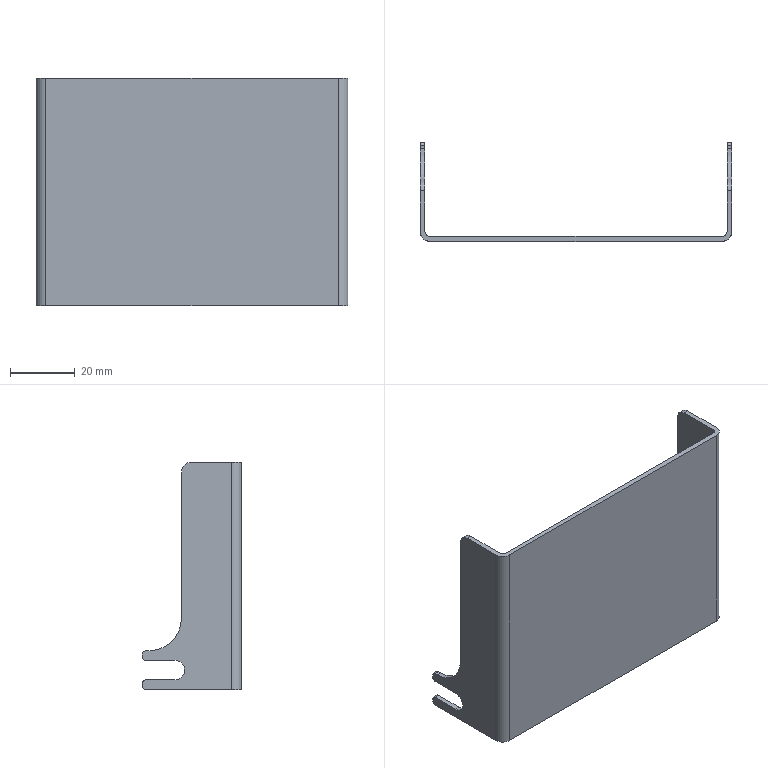Part | NX | features BREP 1 | 1 solid | 38 faces | box 96 x 30.5 x 70 mm | volume 13713 mm3 | plane 20 | cylinder 18 | commonest cylinder face diameters 2 x8 6 x6 3 x2 20 x2
STEP:
#1=CARTESIAN_POINT('',(-45.,0.,70.));
#2=VERTEX_POINT('',#1);
#3=CARTESIAN_POINT('',(45.,0.,70.));
#4=VERTEX_POINT('',#3);
#5=CARTESIAN_POINT('',(-46.5,0.,70.));
#6=DIRECTION('',(1.,0.,0.));
#7=VECTOR('',#6,1000.);
#8=LINE('',#5,#7);
#9=EDGE_CURVE('',#2,#4,#8,.T.);
#10=ORIENTED_EDGE('',*,*,#9,.T.);
#11=CARTESIAN_POINT('',(45.,0.,0.));
#12=VERTEX_POINT('',#11);
#13=CARTESIAN_POINT('',(45.,0.,70.));
#14=DIRECTION('',(0.,0.,-1.));
#15=VECTOR('',#14,1000.);
#16=LINE('',#13,#15);
#17=EDGE_CURVE('',#4,#12,#16,.T.);
#18=ORIENTED_EDGE('',*,*,#17,.T.);
#19=CARTESIAN_POINT('',(-45.,0.,0.));
#20=VERTEX_POINT('',#19);
#21=CARTESIAN_POINT('',(-46.5,0.,0.));
#22=DIRECTION('',(-1.,0.,0.));
#23=VECTOR('',#22,1000.);
#24=LINE('',#21,#23);
#25=EDGE_CURVE('',#12,#20,#24,.T.);
#26=ORIENTED_EDGE('',*,*,#25,.T.);
#27=CARTESIAN_POINT('',(-45.,0.,70.));
#28=DIRECTION('',(0.,0.,1.));
#29=VECTOR('',#28,1000.);
#30=LINE('',#27,#29);
#31=EDGE_CURVE('',#20,#2,#30,.T.);
#32=ORIENTED_EDGE('',*,*,#31,.T.);
#33=EDGE_LOOP('',(#10,#18,#26,#32));
#34=FACE_BOUND('',#33,.T.);
#35=CARTESIAN_POINT('',(-46.5,0.,70.));
#36=DIRECTION('',(0.,1.,0.));
#37=DIRECTION('',(1.,0.,0.));
#38=AXIS2_PLACEMENT_3D('',#35,#36,#37);
#39=PLANE('',#38);
#40=ADVANCED_FACE('',(#34),#39,.T.);
#41=ORIENTED_EDGE('',*,*,#17,.F.);
#42=CARTESIAN_POINT('',(46.5,1.5,70.));
#43=VERTEX_POINT('',#42);
#44=CARTESIAN_POINT('',(45.,1.5,70.));
#45=DIRECTION('',(0.,0.,-1.));
#46=DIRECTION('',(-1.,0.,0.));
#47=AXIS2_PLACEMENT_3D('',#44,#45,#46);
#48=CIRCLE('',#47,1.5);
#49=EDGE_CURVE('',#43,#4,#48,.T.);
#50=ORIENTED_EDGE('',*,*,#49,.F.);
#51=CARTESIAN_POINT('',(46.5,1.5,0.));
#52=VERTEX_POINT('',#51);
#53=CARTESIAN_POINT('',(46.5,1.5,70.));
#54=DIRECTION('',(0.,0.,1.));
#55=VECTOR('',#54,1000.);
#56=LINE('',#53,#55);
#57=EDGE_CURVE('',#52,#43,#56,.T.);
#58=ORIENTED_EDGE('',*,*,#57,.F.);
#59=CARTESIAN_POINT('',(45.,1.5,0.));
#60=DIRECTION('',(0.,0.,1.));
#61=DIRECTION('',(-1.,0.,0.));
#62=AXIS2_PLACEMENT_3D('',#59,#60,#61);
#63=CIRCLE('',#62,1.5);
#64=EDGE_CURVE('',#12,#52,#63,.T.);
#65=ORIENTED_EDGE('',*,*,#64,.F.);
#66=EDGE_LOOP('',(#41,#50,#58,#65));
#67=FACE_BOUND('',#66,.T.);
#68=CARTESIAN_POINT('',(45.,1.5,70.));
#69=DIRECTION('',(0.,0.,-1.));
#70=DIRECTION('',(1.,0.,0.));
#71=AXIS2_PLACEMENT_3D('',#68,#69,#70);
#72=CYLINDRICAL_SURFACE('',#71,1.5);
#73=ADVANCED_FACE('',(#67),#72,.F.);
#74=CARTESIAN_POINT('',(-45.,-1.5,70.));
#75=VERTEX_POINT('',#74);
#76=CARTESIAN_POINT('',(45.,-1.5,70.));
#77=VERTEX_POINT('',#76);
#78=CARTESIAN_POINT('',(-48.,-1.5,70.));
#79=DIRECTION('',(1.,0.,0.));
#80=VECTOR('',#79,1000.);
#81=LINE('',#78,#80);
#82=EDGE_CURVE('',#75,#77,#81,.T.);
#83=ORIENTED_EDGE('',*,*,#82,.T.);
#84=CARTESIAN_POINT('',(48.,1.5,70.));
#85=VERTEX_POINT('',#84);
#86=CARTESIAN_POINT('',(45.,1.5,70.));
#87=DIRECTION('',(0.,0.,1.));
#88=DIRECTION('',(-1.,0.,0.));
#89=AXIS2_PLACEMENT_3D('',#86,#87,#88);
#90=CIRCLE('',#89,3.);
#91=EDGE_CURVE('',#77,#85,#90,.T.);
#92=ORIENTED_EDGE('',*,*,#91,.T.);
#93=CARTESIAN_POINT('',(48.,14.,70.));
#94=VERTEX_POINT('',#93);
#95=CARTESIAN_POINT('',(48.,-1.5,70.));
#96=DIRECTION('',(0.,1.,0.));
#97=VECTOR('',#96,1000.);
#98=LINE('',#95,#97);
#99=EDGE_CURVE('',#85,#94,#98,.T.);
#100=ORIENTED_EDGE('',*,*,#99,.T.);
#101=CARTESIAN_POINT('',(46.5,14.,70.));
#102=VERTEX_POINT('',#101);
#103=CARTESIAN_POINT('',(46.5,14.,70.));
#104=DIRECTION('',(1.,0.,0.));
#105=VECTOR('',#104,1000.);
#106=LINE('',#103,#105);
#107=EDGE_CURVE('',#102,#94,#106,.T.);
#108=ORIENTED_EDGE('',*,*,#107,.F.);
#109=CARTESIAN_POINT('',(46.5,0.,70.));
#110=DIRECTION('',(0.,1.,0.));
#111=VECTOR('',#110,1000.);
#112=LINE('',#109,#111);
#113=EDGE_CURVE('',#43,#102,#112,.T.);
#114=ORIENTED_EDGE('',*,*,#113,.F.);
#115=ORIENTED_EDGE('',*,*,#49,.T.);
#116=ORIENTED_EDGE('',*,*,#9,.F.);
#117=CARTESIAN_POINT('',(-46.5,1.5,70.));
#118=VERTEX_POINT('',#117);
#119=CARTESIAN_POINT('',(-45.,1.5,70.));
#120=DIRECTION('',(0.,0.,-1.));
#121=DIRECTION('',(-1.,0.,0.));
#122=AXIS2_PLACEMENT_3D('',#119,#120,#121);
#123=CIRCLE('',#122,1.5);
#124=EDGE_CURVE('',#2,#118,#123,.T.);
#125=ORIENTED_EDGE('',*,*,#124,.T.);
#126=CARTESIAN_POINT('',(-46.5,14.,70.));
#127=VERTEX_POINT('',#126);
#128=CARTESIAN_POINT('',(-46.5,17.,70.));
#129=DIRECTION('',(0.,-1.,0.));
#130=VECTOR('',#129,1000.);
#131=LINE('',#128,#130);
#132=EDGE_CURVE('',#127,#118,#131,.T.);
#133=ORIENTED_EDGE('',*,*,#132,.F.);
#134=CARTESIAN_POINT('',(-48.,14.,70.));
#135=VERTEX_POINT('',#134);
#136=CARTESIAN_POINT('',(45.,14.,70.));
#137=DIRECTION('',(1.,0.,0.));
#138=VECTOR('',#137,1000.);
#139=LINE('',#136,#138);
#140=EDGE_CURVE('',#135,#127,#139,.T.);
#141=ORIENTED_EDGE('',*,*,#140,.F.);
#142=CARTESIAN_POINT('',(-48.,1.5,70.));
#143=VERTEX_POINT('',#142);
#144=CARTESIAN_POINT('',(-48.,1.5,70.));
#145=DIRECTION('',(0.,1.,0.));
#146=VECTOR('',#145,1000.);
#147=LINE('',#144,#146);
#148=EDGE_CURVE('',#143,#135,#147,.T.);
#149=ORIENTED_EDGE('',*,*,#148,.F.);
#150=CARTESIAN_POINT('',(-45.,1.5,70.));
#151=DIRECTION('',(0.,0.,1.));
#152=DIRECTION('',(-1.,0.,0.));
#153=AXIS2_PLACEMENT_3D('',#150,#151,#152);
#154=CIRCLE('',#153,3.);
#155=EDGE_CURVE('',#143,#75,#154,.T.);
#156=ORIENTED_EDGE('',*,*,#155,.T.);
#157=EDGE_LOOP('',(#83,#92,#100,#108,#114,#115,#116,#125,#133,#141,#149,#156));
#158=FACE_BOUND('',#157,.T.);
#159=CARTESIAN_POINT('',(-48.,1.5,70.));
#160=DIRECTION('',(0.,0.,1.));
#161=DIRECTION('',(-1.,0.,0.));
#162=AXIS2_PLACEMENT_3D('',#159,#160,#161);
#163=PLANE('',#162);
#164=ADVANCED_FACE('',(#158),#163,.T.);
#165=CARTESIAN_POINT('',(-46.5,1.5,0.));
#166=VERTEX_POINT('',#165);
#167=CARTESIAN_POINT('',(-46.5,1.5,70.));
#168=DIRECTION('',(0.,0.,-1.));
#169=VECTOR('',#168,1000.);
#170=LINE('',#167,#169);
#171=EDGE_CURVE('',#118,#166,#170,.T.);
#172=ORIENTED_EDGE('',*,*,#171,.F.);
#173=ORIENTED_EDGE('',*,*,#124,.F.);
#174=ORIENTED_EDGE('',*,*,#31,.F.);
#175=CARTESIAN_POINT('',(-45.,1.5,0.));
#176=DIRECTION('',(0.,0.,1.));
#177=DIRECTION('',(-1.,0.,0.));
#178=AXIS2_PLACEMENT_3D('',#175,#176,#177);
#179=CIRCLE('',#178,1.5);
#180=EDGE_CURVE('',#166,#20,#179,.T.);
#181=ORIENTED_EDGE('',*,*,#180,.F.);
#182=EDGE_LOOP('',(#172,#173,#174,#181));
#183=FACE_BOUND('',#182,.T.);
#184=CARTESIAN_POINT('',(-45.,1.5,70.));
#185=DIRECTION('',(0.,0.,-1.));
#186=DIRECTION('',(1.,0.,0.));
#187=AXIS2_PLACEMENT_3D('',#184,#185,#186);
#188=CYLINDRICAL_SURFACE('',#187,1.5);
#189=ADVANCED_FACE('',(#183),#188,.F.);
#190=CARTESIAN_POINT('',(45.,-1.5,0.));
#191=VERTEX_POINT('',#190);
#192=CARTESIAN_POINT('',(-45.,-1.5,0.));
#193=VERTEX_POINT('',#192);
#194=CARTESIAN_POINT('',(48.,-1.5,0.));
#195=DIRECTION('',(-1.,0.,0.));
#196=VECTOR('',#195,1000.);
#197=LINE('',#194,#196);
#198=EDGE_CURVE('',#191,#193,#197,.T.);
#199=ORIENTED_EDGE('',*,*,#198,.T.);
#200=CARTESIAN_POINT('',(-48.,1.5,0.));
#201=VERTEX_POINT('',#200);
#202=CARTESIAN_POINT('',(-45.,1.5,0.));
#203=DIRECTION('',(0.,0.,-1.));
#204=DIRECTION('',(-1.,0.,0.));
#205=AXIS2_PLACEMENT_3D('',#202,#203,#204);
#206=CIRCLE('',#205,3.);
#207=EDGE_CURVE('',#193,#201,#206,.T.);
#208=ORIENTED_EDGE('',*,*,#207,.T.);
#209=CARTESIAN_POINT('',(-48.,28.,0.));
#210=VERTEX_POINT('',#209);
#211=CARTESIAN_POINT('',(-48.,-1.5,0.));
#212=DIRECTION('',(0.,1.,0.));
#213=VECTOR('',#212,1000.);
#214=LINE('',#211,#213);
#215=EDGE_CURVE('',#201,#210,#214,.T.);
#216=ORIENTED_EDGE('',*,*,#215,.T.);
#217=CARTESIAN_POINT('',(-46.5,28.,0.));
#218=VERTEX_POINT('',#217);
#219=CARTESIAN_POINT('',(-29.529,28.,0.));
#220=DIRECTION('',(-1.,0.,0.));
#221=VECTOR('',#220,1000.);
#222=LINE('',#219,#221);
#223=EDGE_CURVE('',#218,#210,#222,.T.);
#224=ORIENTED_EDGE('',*,*,#223,.F.);
#225=CARTESIAN_POINT('',(-46.5,17.,0.));
#226=DIRECTION('',(0.,1.,0.));
#227=VECTOR('',#226,1000.);
#228=LINE('',#225,#227);
#229=EDGE_CURVE('',#166,#218,#228,.T.);
#230=ORIENTED_EDGE('',*,*,#229,.F.);
#231=ORIENTED_EDGE('',*,*,#180,.T.);
#232=ORIENTED_EDGE('',*,*,#25,.F.);
#233=ORIENTED_EDGE('',*,*,#64,.T.);
#234=CARTESIAN_POINT('',(46.5,28.,0.));
#235=VERTEX_POINT('',#234);
#236=CARTESIAN_POINT('',(46.5,0.,0.));
#237=DIRECTION('',(0.,-1.,0.));
#238=VECTOR('',#237,1000.);
#239=LINE('',#236,#238);
#240=EDGE_CURVE('',#235,#52,#239,.T.);
#241=ORIENTED_EDGE('',*,*,#240,.F.);
#242=CARTESIAN_POINT('',(48.,28.,0.));
#243=VERTEX_POINT('',#242);
#244=CARTESIAN_POINT('',(45.,28.,0.));
#245=DIRECTION('',(1.,0.,0.));
#246=VECTOR('',#245,1000.);
#247=LINE('',#244,#246);
#248=EDGE_CURVE('',#235,#243,#247,.T.);
#249=ORIENTED_EDGE('',*,*,#248,.T.);
#250=CARTESIAN_POINT('',(48.,1.5,0.));
#251=VERTEX_POINT('',#250);
#252=CARTESIAN_POINT('',(48.,1.5,0.));
#253=DIRECTION('',(0.,-1.,0.));
#254=VECTOR('',#253,1000.);
#255=LINE('',#252,#254);
#256=EDGE_CURVE('',#243,#251,#255,.T.);
#257=ORIENTED_EDGE('',*,*,#256,.T.);
#258=CARTESIAN_POINT('',(45.,1.5,0.));
#259=DIRECTION('',(0.,0.,-1.));
#260=DIRECTION('',(-1.,0.,0.));
#261=AXIS2_PLACEMENT_3D('',#258,#259,#260);
#262=CIRCLE('',#261,3.);
#263=EDGE_CURVE('',#251,#191,#262,.T.);
#264=ORIENTED_EDGE('',*,*,#263,.T.);
#265=EDGE_LOOP('',(#199,#208,#216,#224,#230,#231,#232,#233,#241,#249,#257,#264));
#266=FACE_BOUND('',#265,.T.);
#267=CARTESIAN_POINT('',(48.,1.5,0.));
#268=DIRECTION('',(0.,0.,-1.));
#269=DIRECTION('',(1.,0.,0.));
#270=AXIS2_PLACEMENT_3D('',#267,#268,#269);
#271=PLANE('',#270);
#272=ADVANCED_FACE('',(#266),#271,.T.);
#273=CARTESIAN_POINT('',(46.5,27.,12.));
#274=VERTEX_POINT('',#273);
#275=CARTESIAN_POINT('',(46.5,28.,12.));
#276=VERTEX_POINT('',#275);
#277=CARTESIAN_POINT('',(46.5,0.,12.));
#278=DIRECTION('',(0.,1.,0.));
#279=VECTOR('',#278,1000.);
#280=LINE('',#277,#279);
#281=EDGE_CURVE('',#274,#276,#280,.T.);
#282=ORIENTED_EDGE('',*,*,#281,.T.);
#283=CARTESIAN_POINT('',(46.5,29.,11.));
#284=VERTEX_POINT('',#283);
#285=CARTESIAN_POINT('',(46.5,28.,11.));
#286=DIRECTION('',(-1.,0.,0.));
#287=DIRECTION('',(0.,0.,-1.));
#288=AXIS2_PLACEMENT_3D('',#285,#286,#287);
#289=CIRCLE('',#288,1.);
#290=EDGE_CURVE('',#276,#284,#289,.T.);
#291=ORIENTED_EDGE('',*,*,#290,.T.);
#292=CARTESIAN_POINT('',(46.5,29.,10.));
#293=VERTEX_POINT('',#292);
#294=CARTESIAN_POINT('',(46.5,29.,70.));
#295=DIRECTION('',(0.,0.,-1.));
#296=VECTOR('',#295,1000.);
#297=LINE('',#294,#296);
#298=EDGE_CURVE('',#284,#293,#297,.T.);
#299=ORIENTED_EDGE('',*,*,#298,.T.);
#300=CARTESIAN_POINT('',(46.5,28.,9.));
#301=VERTEX_POINT('',#300);
#302=CARTESIAN_POINT('',(46.5,28.,10.));
#303=DIRECTION('',(-1.,0.,0.));
#304=DIRECTION('',(0.,0.,1.));
#305=AXIS2_PLACEMENT_3D('',#302,#303,#304);
#306=CIRCLE('',#305,1.);
#307=EDGE_CURVE('',#293,#301,#306,.T.);
#308=ORIENTED_EDGE('',*,*,#307,.T.);
#309=CARTESIAN_POINT('',(46.5,19.,9.));
#310=VERTEX_POINT('',#309);
#311=CARTESIAN_POINT('',(46.5,0.,9.));
#312=DIRECTION('',(0.,-1.,0.));
#313=VECTOR('',#312,1000.);
#314=LINE('',#311,#313);
#315=EDGE_CURVE('',#301,#310,#314,.T.);
#316=ORIENTED_EDGE('',*,*,#315,.T.);
#317=CARTESIAN_POINT('',(46.5,19.,3.));
#318=VERTEX_POINT('',#317);
#319=CARTESIAN_POINT('',(46.5,19.,6.));
#320=DIRECTION('',(1.,0.,0.));
#321=DIRECTION('',(0.,0.,-1.));
#322=AXIS2_PLACEMENT_3D('',#319,#320,#321);
#323=CIRCLE('',#322,3.);
#324=EDGE_CURVE('',#310,#318,#323,.T.);
#325=ORIENTED_EDGE('',*,*,#324,.T.);
#326=CARTESIAN_POINT('',(46.5,28.,3.));
#327=VERTEX_POINT('',#326);
#328=CARTESIAN_POINT('',(46.5,0.,3.));
#329=DIRECTION('',(0.,1.,0.));
#330=VECTOR('',#329,1000.);
#331=LINE('',#328,#330);
#332=EDGE_CURVE('',#318,#327,#331,.T.);
#333=ORIENTED_EDGE('',*,*,#332,.T.);
#334=CARTESIAN_POINT('',(46.5,29.,2.));
#335=VERTEX_POINT('',#334);
#336=CARTESIAN_POINT('',(46.5,28.,2.));
#337=DIRECTION('',(-1.,0.,0.));
#338=DIRECTION('',(0.,0.,-1.));
#339=AXIS2_PLACEMENT_3D('',#336,#337,#338);
#340=CIRCLE('',#339,1.);
#341=EDGE_CURVE('',#327,#335,#340,.T.);
#342=ORIENTED_EDGE('',*,*,#341,.T.);
#343=CARTESIAN_POINT('',(46.5,29.,1.));
#344=VERTEX_POINT('',#343);
#345=CARTESIAN_POINT('',(46.5,29.,70.));
#346=DIRECTION('',(0.,0.,-1.));
#347=VECTOR('',#346,1000.);
#348=LINE('',#345,#347);
#349=EDGE_CURVE('',#335,#344,#348,.T.);
#350=ORIENTED_EDGE('',*,*,#349,.T.);
#351=CARTESIAN_POINT('',(46.5,28.,1.));
#352=DIRECTION('',(-1.,0.,0.));
#353=DIRECTION('',(0.,0.,-1.));
#354=AXIS2_PLACEMENT_3D('',#351,#352,#353);
#355=CIRCLE('',#354,1.);
#356=EDGE_CURVE('',#344,#235,#355,.T.);
#357=ORIENTED_EDGE('',*,*,#356,.T.);
#358=ORIENTED_EDGE('',*,*,#240,.T.);
#359=ORIENTED_EDGE('',*,*,#57,.T.);
#360=ORIENTED_EDGE('',*,*,#113,.T.);
#361=CARTESIAN_POINT('',(46.5,17.,67.));
#362=VERTEX_POINT('',#361);
#363=CARTESIAN_POINT('',(46.5,14.,67.));
#364=DIRECTION('',(-1.,0.,0.));
#365=DIRECTION('',(0.,0.,-1.));
#366=AXIS2_PLACEMENT_3D('',#363,#364,#365);
#367=CIRCLE('',#366,3.);
#368=EDGE_CURVE('',#102,#362,#367,.T.);
#369=ORIENTED_EDGE('',*,*,#368,.T.);
#370=CARTESIAN_POINT('',(46.5,17.,22.));
#371=VERTEX_POINT('',#370);
#372=CARTESIAN_POINT('',(46.5,17.,70.));
#373=DIRECTION('',(0.,0.,-1.));
#374=VECTOR('',#373,1000.);
#375=LINE('',#372,#374);
#376=EDGE_CURVE('',#362,#371,#375,.T.);
#377=ORIENTED_EDGE('',*,*,#376,.T.);
#378=CARTESIAN_POINT('',(46.5,27.,22.));
#379=DIRECTION('',(1.,0.,0.));
#380=DIRECTION('',(0.,0.,1.));
#381=AXIS2_PLACEMENT_3D('',#378,#379,#380);
#382=CIRCLE('',#381,10.);
#383=EDGE_CURVE('',#371,#274,#382,.T.);
#384=ORIENTED_EDGE('',*,*,#383,.T.);
#385=EDGE_LOOP('',(#282,#291,#299,#308,#316,#325,#333,#342,#350,#357,#358,#359,#360,#369,#377,#384));
#386=FACE_BOUND('',#385,.T.);
#387=CARTESIAN_POINT('',(46.5,0.,70.));
#388=DIRECTION('',(-1.,0.,0.));
#389=DIRECTION('',(0.,0.,-1.));
#390=AXIS2_PLACEMENT_3D('',#387,#388,#389);
#391=PLANE('',#390);
#392=ADVANCED_FACE('',(#386),#391,.T.);
#393=CARTESIAN_POINT('',(45.,-1.5,70.));
#394=DIRECTION('',(0.,0.,-1.));
#395=VECTOR('',#394,1000.);
#396=LINE('',#393,#395);
#397=EDGE_CURVE('',#77,#191,#396,.T.);
#398=ORIENTED_EDGE('',*,*,#397,.F.);
#399=ORIENTED_EDGE('',*,*,#82,.F.);
#400=CARTESIAN_POINT('',(-45.,-1.5,70.));
#401=DIRECTION('',(0.,0.,1.));
#402=VECTOR('',#401,1000.);
#403=LINE('',#400,#402);
#404=EDGE_CURVE('',#193,#75,#403,.T.);
#405=ORIENTED_EDGE('',*,*,#404,.F.);
#406=ORIENTED_EDGE('',*,*,#198,.F.);
#407=EDGE_LOOP('',(#398,#399,#405,#406));
#408=FACE_BOUND('',#407,.T.);
#409=CARTESIAN_POINT('',(-46.5,-1.5,70.));
#410=DIRECTION('',(0.,1.,0.));
#411=DIRECTION('',(1.,0.,0.));
#412=AXIS2_PLACEMENT_3D('',#409,#410,#411);
#413=PLANE('',#412);
#414=ADVANCED_FACE('',(#408),#413,.F.);
#415=ORIENTED_EDGE('',*,*,#229,.T.);
#416=CARTESIAN_POINT('',(-46.5,29.,1.));
#417=VERTEX_POINT('',#416);
#418=CARTESIAN_POINT('',(-46.5,28.,1.));
#419=DIRECTION('',(1.,0.,0.));
#420=DIRECTION('',(0.,0.,1.));
#421=AXIS2_PLACEMENT_3D('',#418,#419,#420);
#422=CIRCLE('',#421,1.);
#423=EDGE_CURVE('',#218,#417,#422,.T.);
#424=ORIENTED_EDGE('',*,*,#423,.T.);
#425=CARTESIAN_POINT('',(-46.5,29.,2.));
#426=VERTEX_POINT('',#425);
#427=CARTESIAN_POINT('',(-46.5,29.,70.));
#428=DIRECTION('',(0.,0.,1.));
#429=VECTOR('',#428,1000.);
#430=LINE('',#427,#429);
#431=EDGE_CURVE('',#417,#426,#430,.T.);
#432=ORIENTED_EDGE('',*,*,#431,.T.);
#433=CARTESIAN_POINT('',(-46.5,28.,3.));
#434=VERTEX_POINT('',#433);
#435=CARTESIAN_POINT('',(-46.5,28.,2.));
#436=DIRECTION('',(1.,0.,0.));
#437=DIRECTION('',(0.,0.,1.));
#438=AXIS2_PLACEMENT_3D('',#435,#436,#437);
#439=CIRCLE('',#438,1.);
#440=EDGE_CURVE('',#426,#434,#439,.T.);
#441=ORIENTED_EDGE('',*,*,#440,.T.);
#442=CARTESIAN_POINT('',(-46.5,19.,3.));
#443=VERTEX_POINT('',#442);
#444=CARTESIAN_POINT('',(-46.5,17.,3.));
#445=DIRECTION('',(0.,-1.,0.));
#446=VECTOR('',#445,1000.);
#447=LINE('',#444,#446);
#448=EDGE_CURVE('',#434,#443,#447,.T.);
#449=ORIENTED_EDGE('',*,*,#448,.T.);
#450=CARTESIAN_POINT('',(-46.5,19.,9.));
#451=VERTEX_POINT('',#450);
#452=CARTESIAN_POINT('',(-46.5,19.,6.));
#453=DIRECTION('',(-1.,0.,0.));
#454=DIRECTION('',(0.,0.,-1.));
#455=AXIS2_PLACEMENT_3D('',#452,#453,#454);
#456=CIRCLE('',#455,3.);
#457=EDGE_CURVE('',#443,#451,#456,.T.);
#458=ORIENTED_EDGE('',*,*,#457,.T.);
#459=CARTESIAN_POINT('',(-46.5,28.,9.));
#460=VERTEX_POINT('',#459);
#461=CARTESIAN_POINT('',(-46.5,17.,9.));
#462=DIRECTION('',(0.,1.,0.));
#463=VECTOR('',#462,1000.);
#464=LINE('',#461,#463);
#465=EDGE_CURVE('',#451,#460,#464,.T.);
#466=ORIENTED_EDGE('',*,*,#465,.T.);
#467=CARTESIAN_POINT('',(-46.5,29.,10.));
#468=VERTEX_POINT('',#467);
#469=CARTESIAN_POINT('',(-46.5,28.,10.));
#470=DIRECTION('',(1.,0.,0.));
#471=DIRECTION('',(0.,0.,1.));
#472=AXIS2_PLACEMENT_3D('',#469,#470,#471);
#473=CIRCLE('',#472,1.);
#474=EDGE_CURVE('',#460,#468,#473,.T.);
#475=ORIENTED_EDGE('',*,*,#474,.T.);
#476=CARTESIAN_POINT('',(-46.5,29.,11.));
#477=VERTEX_POINT('',#476);
#478=CARTESIAN_POINT('',(-46.5,29.,70.));
#479=DIRECTION('',(0.,0.,1.));
#480=VECTOR('',#479,1000.);
#481=LINE('',#478,#480);
#482=EDGE_CURVE('',#468,#477,#481,.T.);
#483=ORIENTED_EDGE('',*,*,#482,.T.);
#484=CARTESIAN_POINT('',(-46.5,28.,12.));
#485=VERTEX_POINT('',#484);
#486=CARTESIAN_POINT('',(-46.5,28.,11.));
#487=DIRECTION('',(1.,0.,0.));
#488=DIRECTION('',(0.,0.,1.));
#489=AXIS2_PLACEMENT_3D('',#486,#487,#488);
#490=CIRCLE('',#489,1.);
#491=EDGE_CURVE('',#477,#485,#490,.T.);
#492=ORIENTED_EDGE('',*,*,#491,.T.);
#493=CARTESIAN_POINT('',(-46.5,27.,12.));
#494=VERTEX_POINT('',#493);
#495=CARTESIAN_POINT('',(-46.5,17.,12.));
#496=DIRECTION('',(0.,-1.,0.));
#497=VECTOR('',#496,1000.);
#498=LINE('',#495,#497);
#499=EDGE_CURVE('',#485,#494,#498,.T.);
#500=ORIENTED_EDGE('',*,*,#499,.T.);
#501=CARTESIAN_POINT('',(-46.5,17.,22.));
#502=VERTEX_POINT('',#501);
#503=CARTESIAN_POINT('',(-46.5,27.,22.));
#504=DIRECTION('',(-1.,0.,0.));
#505=DIRECTION('',(0.,0.,-1.));
#506=AXIS2_PLACEMENT_3D('',#503,#504,#505);
#507=CIRCLE('',#506,10.);
#508=EDGE_CURVE('',#494,#502,#507,.T.);
#509=ORIENTED_EDGE('',*,*,#508,.T.);
#510=CARTESIAN_POINT('',(-46.5,17.,67.));
#511=VERTEX_POINT('',#510);
#512=CARTESIAN_POINT('',(-46.5,17.,70.));
#513=DIRECTION('',(0.,0.,1.));
#514=VECTOR('',#513,1000.);
#515=LINE('',#512,#514);
#516=EDGE_CURVE('',#502,#511,#515,.T.);
#517=ORIENTED_EDGE('',*,*,#516,.T.);
#518=CARTESIAN_POINT('',(-46.5,14.,67.));
#519=DIRECTION('',(1.,0.,0.));
#520=DIRECTION('',(0.,0.,1.));
#521=AXIS2_PLACEMENT_3D('',#518,#519,#520);
#522=CIRCLE('',#521,3.);
#523=EDGE_CURVE('',#511,#127,#522,.T.);
#524=ORIENTED_EDGE('',*,*,#523,.T.);
#525=ORIENTED_EDGE('',*,*,#132,.T.);
#526=ORIENTED_EDGE('',*,*,#171,.T.);
#527=EDGE_LOOP('',(#415,#424,#432,#441,#449,#458,#466,#475,#483,#492,#500,#509,#517,#524,#525,#526));
#528=FACE_BOUND('',#527,.T.);
#529=CARTESIAN_POINT('',(-46.5,17.,70.));
#530=DIRECTION('',(1.,0.,0.));
#531=DIRECTION('',(0.,0.,1.));
#532=AXIS2_PLACEMENT_3D('',#529,#530,#531);
#533=PLANE('',#532);
#534=ADVANCED_FACE('',(#528),#533,.T.);
#535=ORIENTED_EDGE('',*,*,#91,.F.);
#536=ORIENTED_EDGE('',*,*,#397,.T.);
#537=ORIENTED_EDGE('',*,*,#263,.F.);
#538=CARTESIAN_POINT('',(48.,1.5,70.));
#539=DIRECTION('',(0.,0.,1.));
#540=VECTOR('',#539,1000.);
#541=LINE('',#538,#540);
#542=EDGE_CURVE('',#251,#85,#541,.T.);
#543=ORIENTED_EDGE('',*,*,#542,.T.);
#544=EDGE_LOOP('',(#535,#536,#537,#543));
#545=FACE_BOUND('',#544,.T.);
#546=CARTESIAN_POINT('',(45.,1.5,70.));
#547=DIRECTION('',(0.,0.,-1.));
#548=DIRECTION('',(1.,0.,0.));
#549=AXIS2_PLACEMENT_3D('',#546,#547,#548);
#550=CYLINDRICAL_SURFACE('',#549,3.);
#551=ADVANCED_FACE('',(#545),#550,.T.);
#552=CARTESIAN_POINT('',(48.,28.,12.));
#553=VERTEX_POINT('',#552);
#554=CARTESIAN_POINT('',(48.,29.,11.));
#555=VERTEX_POINT('',#554);
#556=CARTESIAN_POINT('',(48.,28.,11.));
#557=DIRECTION('',(-1.,0.,0.));
#558=DIRECTION('',(0.,0.,-1.));
#559=AXIS2_PLACEMENT_3D('',#556,#557,#558);
#560=CIRCLE('',#559,1.);
#561=EDGE_CURVE('',#553,#555,#560,.T.);
#562=ORIENTED_EDGE('',*,*,#561,.T.);
#563=CARTESIAN_POINT('',(46.5,29.,11.));
#564=DIRECTION('',(-1.,0.,0.));
#565=VECTOR('',#564,1000.);
#566=LINE('',#563,#565);
#567=EDGE_CURVE('',#555,#284,#566,.T.);
#568=ORIENTED_EDGE('',*,*,#567,.T.);
#569=ORIENTED_EDGE('',*,*,#290,.F.);
#570=CARTESIAN_POINT('',(46.5,28.,12.));
#571=DIRECTION('',(1.,0.,0.));
#572=VECTOR('',#571,1000.);
#573=LINE('',#570,#572);
#574=EDGE_CURVE('',#276,#553,#573,.T.);
#575=ORIENTED_EDGE('',*,*,#574,.T.);
#576=EDGE_LOOP('',(#562,#568,#569,#575));
#577=FACE_BOUND('',#576,.T.);
#578=CARTESIAN_POINT('',(46.5,28.,11.));
#579=DIRECTION('',(1.,0.,0.));
#580=DIRECTION('',(0.,0.,1.));
#581=AXIS2_PLACEMENT_3D('',#578,#579,#580);
#582=CYLINDRICAL_SURFACE('',#581,1.);
#583=ADVANCED_FACE('',(#577),#582,.T.);
#584=ORIENTED_EDGE('',*,*,#281,.F.);
#585=CARTESIAN_POINT('',(48.,27.,12.));
#586=VERTEX_POINT('',#585);
#587=CARTESIAN_POINT('',(46.5,27.,12.));
#588=DIRECTION('',(1.,0.,0.));
#589=VECTOR('',#588,1000.);
#590=LINE('',#587,#589);
#591=EDGE_CURVE('',#274,#586,#590,.T.);
#592=ORIENTED_EDGE('',*,*,#591,.T.);
#593=CARTESIAN_POINT('',(48.,29.,12.));
#594=DIRECTION('',(0.,1.,0.));
#595=VECTOR('',#594,1000.);
#596=LINE('',#593,#595);
#597=EDGE_CURVE('',#586,#553,#596,.T.);
#598=ORIENTED_EDGE('',*,*,#597,.T.);
#599=ORIENTED_EDGE('',*,*,#574,.F.);
#600=EDGE_LOOP('',(#584,#592,#598,#599));
#601=FACE_BOUND('',#600,.T.);
#602=CARTESIAN_POINT('',(46.5,29.,12.));
#603=DIRECTION('',(0.,0.,1.));
#604=DIRECTION('',(0.,1.,0.));
#605=AXIS2_PLACEMENT_3D('',#602,#603,#604);
#606=PLANE('',#605);
#607=ADVANCED_FACE('',(#601),#606,.T.);
#608=CARTESIAN_POINT('',(48.,17.,22.));
#609=VERTEX_POINT('',#608);
#610=CARTESIAN_POINT('',(46.5,17.,22.));
#611=DIRECTION('',(-1.,0.,0.));
#612=VECTOR('',#611,1000.);
#613=LINE('',#610,#612);
#614=EDGE_CURVE('',#609,#371,#613,.T.);
#615=ORIENTED_EDGE('',*,*,#614,.F.);
#616=CARTESIAN_POINT('',(48.,27.,22.));
#617=DIRECTION('',(-1.,0.,0.));
#618=DIRECTION('',(0.,0.,1.));
#619=AXIS2_PLACEMENT_3D('',#616,#617,#618);
#620=CIRCLE('',#619,10.);
#621=EDGE_CURVE('',#586,#609,#620,.T.);
#622=ORIENTED_EDGE('',*,*,#621,.F.);
#623=ORIENTED_EDGE('',*,*,#591,.F.);
#624=ORIENTED_EDGE('',*,*,#383,.F.);
#625=EDGE_LOOP('',(#615,#622,#623,#624));
#626=FACE_BOUND('',#625,.T.);
#627=CARTESIAN_POINT('',(46.5,27.,22.));
#628=DIRECTION('',(-1.,0.,0.));
#629=DIRECTION('',(0.,0.,-1.));
#630=AXIS2_PLACEMENT_3D('',#627,#628,#629);
#631=CYLINDRICAL_SURFACE('',#630,10.);
#632=ADVANCED_FACE('',(#626),#631,.F.);
#633=CARTESIAN_POINT('',(48.,17.,67.));
#634=VERTEX_POINT('',#633);
#635=CARTESIAN_POINT('',(48.,17.,70.));
#636=DIRECTION('',(0.,0.,-1.));
#637=VECTOR('',#636,1000.);
#638=LINE('',#635,#637);
#639=EDGE_CURVE('',#634,#609,#638,.T.);
#640=ORIENTED_EDGE('',*,*,#639,.T.);
#641=ORIENTED_EDGE('',*,*,#614,.T.);
#642=ORIENTED_EDGE('',*,*,#376,.F.);
#643=CARTESIAN_POINT('',(46.5,17.,67.));
#644=DIRECTION('',(1.,0.,0.));
#645=VECTOR('',#644,1000.);
#646=LINE('',#643,#645);
#647=EDGE_CURVE('',#362,#634,#646,.T.);
#648=ORIENTED_EDGE('',*,*,#647,.T.);
#649=EDGE_LOOP('',(#640,#641,#642,#648));
#650=FACE_BOUND('',#649,.T.);
#651=CARTESIAN_POINT('',(46.5,17.,70.));
#652=DIRECTION('',(0.,1.,0.));
#653=DIRECTION('',(0.,0.,-1.));
#654=AXIS2_PLACEMENT_3D('',#651,#652,#653);
#655=PLANE('',#654);
#656=ADVANCED_FACE('',(#650),#655,.T.);
#657=CARTESIAN_POINT('',(48.,14.,67.));
#658=DIRECTION('',(-1.,0.,0.));
#659=DIRECTION('',(0.,0.,-1.));
#660=AXIS2_PLACEMENT_3D('',#657,#658,#659);
#661=CIRCLE('',#660,3.);
#662=EDGE_CURVE('',#94,#634,#661,.T.);
#663=ORIENTED_EDGE('',*,*,#662,.T.);
#664=ORIENTED_EDGE('',*,*,#647,.F.);
#665=ORIENTED_EDGE('',*,*,#368,.F.);
#666=ORIENTED_EDGE('',*,*,#107,.T.);
#667=EDGE_LOOP('',(#663,#664,#665,#666));
#668=FACE_BOUND('',#667,.T.);
#669=CARTESIAN_POINT('',(46.5,14.,67.));
#670=DIRECTION('',(1.,0.,0.));
#671=DIRECTION('',(0.,0.,1.));
#672=AXIS2_PLACEMENT_3D('',#669,#670,#671);
#673=CYLINDRICAL_SURFACE('',#672,3.);
#674=ADVANCED_FACE('',(#668),#673,.T.);
#675=CARTESIAN_POINT('',(48.,29.,1.));
#676=VERTEX_POINT('',#675);
#677=CARTESIAN_POINT('',(48.,28.,1.));
#678=DIRECTION('',(-1.,0.,0.));
#679=DIRECTION('',(0.,0.,-1.));
#680=AXIS2_PLACEMENT_3D('',#677,#678,#679);
#681=CIRCLE('',#680,1.);
#682=EDGE_CURVE('',#676,#243,#681,.T.);
#683=ORIENTED_EDGE('',*,*,#682,.T.);
#684=ORIENTED_EDGE('',*,*,#248,.F.);
#685=ORIENTED_EDGE('',*,*,#356,.F.);
#686=CARTESIAN_POINT('',(45.,29.,1.));
#687=DIRECTION('',(1.,0.,0.));
#688=VECTOR('',#687,1000.);
#689=LINE('',#686,#688);
#690=EDGE_CURVE('',#344,#676,#689,.T.);
#691=ORIENTED_EDGE('',*,*,#690,.T.);
#692=EDGE_LOOP('',(#683,#684,#685,#691));
#693=FACE_BOUND('',#692,.T.);
#694=CARTESIAN_POINT('',(45.,28.,1.));
#695=DIRECTION('',(1.,0.,0.));
#696=DIRECTION('',(0.,0.,1.));
#697=AXIS2_PLACEMENT_3D('',#694,#695,#696);
#698=CYLINDRICAL_SURFACE('',#697,1.);
#699=ADVANCED_FACE('',(#693),#698,.T.);
#700=CARTESIAN_POINT('',(48.,29.,2.));
#701=VERTEX_POINT('',#700);
#702=CARTESIAN_POINT('',(48.,29.,0.));
#703=DIRECTION('',(0.,0.,-1.));
#704=VECTOR('',#703,1000.);
#705=LINE('',#702,#704);
#706=EDGE_CURVE('',#701,#676,#705,.T.);
#707=ORIENTED_EDGE('',*,*,#706,.T.);
#708=ORIENTED_EDGE('',*,*,#690,.F.);
#709=ORIENTED_EDGE('',*,*,#349,.F.);
#710=CARTESIAN_POINT('',(46.5,29.,2.));
#711=DIRECTION('',(1.,0.,0.));
#712=VECTOR('',#711,1000.);
#713=LINE('',#710,#712);
#714=EDGE_CURVE('',#335,#701,#713,.T.);
#715=ORIENTED_EDGE('',*,*,#714,.T.);
#716=EDGE_LOOP('',(#707,#708,#709,#715));
#717=FACE_BOUND('',#716,.T.);
#718=CARTESIAN_POINT('',(46.5,29.,0.));
#719=DIRECTION('',(0.,1.,0.));
#720=DIRECTION('',(0.,0.,-1.));
#721=AXIS2_PLACEMENT_3D('',#718,#719,#720);
#722=PLANE('',#721);
#723=ADVANCED_FACE('',(#717),#722,.T.);
#724=ORIENTED_EDGE('',*,*,#341,.F.);
#725=CARTESIAN_POINT('',(48.,28.,3.));
#726=VERTEX_POINT('',#725);
#727=CARTESIAN_POINT('',(-48.,28.,3.));
#728=DIRECTION('',(1.,0.,0.));
#729=VECTOR('',#728,1000.);
#730=LINE('',#727,#729);
#731=EDGE_CURVE('',#327,#726,#730,.T.);
#732=ORIENTED_EDGE('',*,*,#731,.T.);
#733=CARTESIAN_POINT('',(48.,28.,2.));
#734=DIRECTION('',(-1.,0.,0.));
#735=DIRECTION('',(0.,0.,-1.));
#736=AXIS2_PLACEMENT_3D('',#733,#734,#735);
#737=CIRCLE('',#736,1.);
#738=EDGE_CURVE('',#726,#701,#737,.T.);
#739=ORIENTED_EDGE('',*,*,#738,.T.);
#740=ORIENTED_EDGE('',*,*,#714,.F.);
#741=EDGE_LOOP('',(#724,#732,#739,#740));
#742=FACE_BOUND('',#741,.T.);
#743=CARTESIAN_POINT('',(-48.,28.,2.));
#744=DIRECTION('',(1.,0.,0.));
#745=DIRECTION('',(0.,0.,1.));
#746=AXIS2_PLACEMENT_3D('',#743,#744,#745);
#747=CYLINDRICAL_SURFACE('',#746,1.);
#748=ADVANCED_FACE('',(#742),#747,.T.);
#749=ORIENTED_EDGE('',*,*,#731,.F.);
#750=ORIENTED_EDGE('',*,*,#332,.F.);
#751=CARTESIAN_POINT('',(48.,19.,3.));
#752=VERTEX_POINT('',#751);
#753=CARTESIAN_POINT('',(-48.,19.,3.));
#754=DIRECTION('',(-1.,0.,0.));
#755=VECTOR('',#754,1000.);
#756=LINE('',#753,#755);
#757=EDGE_CURVE('',#752,#318,#756,.T.);
#758=ORIENTED_EDGE('',*,*,#757,.F.);
#759=CARTESIAN_POINT('',(48.,29.,3.));
#760=DIRECTION('',(0.,-1.,0.));
#761=VECTOR('',#760,1000.);
#762=LINE('',#759,#761);
#763=EDGE_CURVE('',#726,#752,#762,.T.);
#764=ORIENTED_EDGE('',*,*,#763,.F.);
#765=EDGE_LOOP('',(#749,#750,#758,#764));
#766=FACE_BOUND('',#765,.T.);
#767=CARTESIAN_POINT('',(-48.,29.,3.));
#768=DIRECTION('',(0.,0.,-1.));
#769=DIRECTION('',(0.,-1.,0.));
#770=AXIS2_PLACEMENT_3D('',#767,#768,#769);
#771=PLANE('',#770);
#772=ADVANCED_FACE('',(#766),#771,.F.);
#773=CARTESIAN_POINT('',(48.,19.,9.));
#774=VERTEX_POINT('',#773);
#775=CARTESIAN_POINT('',(-48.,19.,9.));
#776=DIRECTION('',(-1.,0.,0.));
#777=VECTOR('',#776,1000.);
#778=LINE('',#775,#777);
#779=EDGE_CURVE('',#774,#310,#778,.T.);
#780=ORIENTED_EDGE('',*,*,#779,.F.);
#781=CARTESIAN_POINT('',(48.,19.,6.));
#782=DIRECTION('',(-1.,0.,0.));
#783=DIRECTION('',(0.,0.,-1.));
#784=AXIS2_PLACEMENT_3D('',#781,#782,#783);
#785=CIRCLE('',#784,3.);
#786=EDGE_CURVE('',#752,#774,#785,.T.);
#787=ORIENTED_EDGE('',*,*,#786,.F.);
#788=ORIENTED_EDGE('',*,*,#757,.T.);
#789=ORIENTED_EDGE('',*,*,#324,.F.);
#790=EDGE_LOOP('',(#780,#787,#788,#789));
#791=FACE_BOUND('',#790,.T.);
#792=CARTESIAN_POINT('',(-48.,19.,6.));
#793=DIRECTION('',(1.,0.,0.));
#794=DIRECTION('',(0.,0.,1.));
#795=AXIS2_PLACEMENT_3D('',#792,#793,#794);
#796=CYLINDRICAL_SURFACE('',#795,3.);
#797=ADVANCED_FACE('',(#791),#796,.F.);
#798=CARTESIAN_POINT('',(48.,28.,9.));
#799=VERTEX_POINT('',#798);
#800=CARTESIAN_POINT('',(-48.,28.,9.));
#801=DIRECTION('',(-1.,0.,0.));
#802=VECTOR('',#801,1000.);
#803=LINE('',#800,#802);
#804=EDGE_CURVE('',#799,#301,#803,.T.);
#805=ORIENTED_EDGE('',*,*,#804,.F.);
#806=CARTESIAN_POINT('',(48.,29.,9.));
#807=DIRECTION('',(0.,1.,0.));
#808=VECTOR('',#807,1000.);
#809=LINE('',#806,#808);
#810=EDGE_CURVE('',#774,#799,#809,.T.);
#811=ORIENTED_EDGE('',*,*,#810,.F.);
#812=ORIENTED_EDGE('',*,*,#779,.T.);
#813=ORIENTED_EDGE('',*,*,#315,.F.);
#814=EDGE_LOOP('',(#805,#811,#812,#813));
#815=FACE_BOUND('',#814,.T.);
#816=CARTESIAN_POINT('',(-48.,29.,9.));
#817=DIRECTION('',(0.,0.,1.));
#818=DIRECTION('',(0.,1.,0.));
#819=AXIS2_PLACEMENT_3D('',#816,#817,#818);
#820=PLANE('',#819);
#821=ADVANCED_FACE('',(#815),#820,.F.);
#822=CARTESIAN_POINT('',(48.,29.,10.));
#823=VERTEX_POINT('',#822);
#824=CARTESIAN_POINT('',(48.,28.,10.));
#825=DIRECTION('',(-1.,0.,0.));
#826=DIRECTION('',(0.,0.,1.));
#827=AXIS2_PLACEMENT_3D('',#824,#825,#826);
#828=CIRCLE('',#827,1.);
#829=EDGE_CURVE('',#823,#799,#828,.T.);
#830=ORIENTED_EDGE('',*,*,#829,.T.);
#831=ORIENTED_EDGE('',*,*,#804,.T.);
#832=ORIENTED_EDGE('',*,*,#307,.F.);
#833=CARTESIAN_POINT('',(-48.,29.,10.));
#834=DIRECTION('',(1.,0.,0.));
#835=VECTOR('',#834,1000.);
#836=LINE('',#833,#835);
#837=EDGE_CURVE('',#293,#823,#836,.T.);
#838=ORIENTED_EDGE('',*,*,#837,.T.);
#839=EDGE_LOOP('',(#830,#831,#832,#838));
#840=FACE_BOUND('',#839,.T.);
#841=CARTESIAN_POINT('',(-48.,28.,10.));
#842=DIRECTION('',(-1.,0.,0.));
#843=DIRECTION('',(0.,0.,-1.));
#844=AXIS2_PLACEMENT_3D('',#841,#842,#843);
#845=CYLINDRICAL_SURFACE('',#844,1.);
#846=ADVANCED_FACE('',(#840),#845,.T.);
#847=ORIENTED_EDGE('',*,*,#298,.F.);
#848=ORIENTED_EDGE('',*,*,#567,.F.);
#849=CARTESIAN_POINT('',(48.,29.,0.));
#850=DIRECTION('',(0.,0.,-1.));
#851=VECTOR('',#850,1000.);
#852=LINE('',#849,#851);
#853=EDGE_CURVE('',#555,#823,#852,.T.);
#854=ORIENTED_EDGE('',*,*,#853,.T.);
#855=ORIENTED_EDGE('',*,*,#837,.F.);
#856=EDGE_LOOP('',(#847,#848,#854,#855));
#857=FACE_BOUND('',#856,.T.);
#858=CARTESIAN_POINT('',(46.5,29.,0.));
#859=DIRECTION('',(0.,1.,0.));
#860=DIRECTION('',(0.,0.,-1.));
#861=AXIS2_PLACEMENT_3D('',#858,#859,#860);
#862=PLANE('',#861);
#863=ADVANCED_FACE('',(#857),#862,.T.);
#864=ORIENTED_EDGE('',*,*,#155,.F.);
#865=CARTESIAN_POINT('',(-48.,1.5,70.));
#866=DIRECTION('',(0.,0.,-1.));
#867=VECTOR('',#866,1000.);
#868=LINE('',#865,#867);
#869=EDGE_CURVE('',#143,#201,#868,.T.);
#870=ORIENTED_EDGE('',*,*,#869,.T.);
#871=ORIENTED_EDGE('',*,*,#207,.F.);
#872=ORIENTED_EDGE('',*,*,#404,.T.);
#873=EDGE_LOOP('',(#864,#870,#871,#872));
#874=FACE_BOUND('',#873,.T.);
#875=CARTESIAN_POINT('',(-45.,1.5,70.));
#876=DIRECTION('',(0.,0.,-1.));
#877=DIRECTION('',(1.,0.,0.));
#878=AXIS2_PLACEMENT_3D('',#875,#876,#877);
#879=CYLINDRICAL_SURFACE('',#878,3.);
#880=ADVANCED_FACE('',(#874),#879,.T.);
#881=CARTESIAN_POINT('',(-48.,29.,1.));
#882=VERTEX_POINT('',#881);
#883=CARTESIAN_POINT('',(-48.,28.,1.));
#884=DIRECTION('',(1.,0.,0.));
#885=DIRECTION('',(0.,0.,1.));
#886=AXIS2_PLACEMENT_3D('',#883,#884,#885);
#887=CIRCLE('',#886,1.);
#888=EDGE_CURVE('',#210,#882,#887,.T.);
#889=ORIENTED_EDGE('',*,*,#888,.T.);
#890=CARTESIAN_POINT('',(-29.529,29.,1.));
#891=DIRECTION('',(1.,0.,0.));
#892=VECTOR('',#891,1000.);
#893=LINE('',#890,#892);
#894=EDGE_CURVE('',#882,#417,#893,.T.);
#895=ORIENTED_EDGE('',*,*,#894,.T.);
#896=ORIENTED_EDGE('',*,*,#423,.F.);
#897=ORIENTED_EDGE('',*,*,#223,.T.);
#898=EDGE_LOOP('',(#889,#895,#896,#897));
#899=FACE_BOUND('',#898,.T.);
#900=CARTESIAN_POINT('',(-29.529,28.,1.));
#901=DIRECTION('',(-1.,0.,0.));
#902=DIRECTION('',(0.,0.,-1.));
#903=AXIS2_PLACEMENT_3D('',#900,#901,#902);
#904=CYLINDRICAL_SURFACE('',#903,1.);
#905=ADVANCED_FACE('',(#899),#904,.T.);
#906=ORIENTED_EDGE('',*,*,#523,.F.);
#907=CARTESIAN_POINT('',(-48.,17.,67.));
#908=VERTEX_POINT('',#907);
#909=CARTESIAN_POINT('',(-48.,17.,67.));
#910=DIRECTION('',(-1.,0.,0.));
#911=VECTOR('',#910,1000.);
#912=LINE('',#909,#911);
#913=EDGE_CURVE('',#511,#908,#912,.T.);
#914=ORIENTED_EDGE('',*,*,#913,.T.);
#915=CARTESIAN_POINT('',(-48.,14.,67.));
#916=DIRECTION('',(1.,0.,0.));
#917=DIRECTION('',(0.,0.,1.));
#918=AXIS2_PLACEMENT_3D('',#915,#916,#917);
#919=CIRCLE('',#918,3.);
#920=EDGE_CURVE('',#908,#135,#919,.T.);
#921=ORIENTED_EDGE('',*,*,#920,.T.);
#922=ORIENTED_EDGE('',*,*,#140,.T.);
#923=EDGE_LOOP('',(#906,#914,#921,#922));
#924=FACE_BOUND('',#923,.T.);
#925=CARTESIAN_POINT('',(-48.,14.,67.));
#926=DIRECTION('',(-1.,0.,0.));
#927=DIRECTION('',(0.,0.,-1.));
#928=AXIS2_PLACEMENT_3D('',#925,#926,#927);
#929=CYLINDRICAL_SURFACE('',#928,3.);
#930=ADVANCED_FACE('',(#924),#929,.T.);
#931=ORIENTED_EDGE('',*,*,#516,.F.);
#932=CARTESIAN_POINT('',(-48.,17.,22.));
#933=VERTEX_POINT('',#932);
#934=CARTESIAN_POINT('',(-48.,17.,22.));
#935=DIRECTION('',(-1.,0.,0.));
#936=VECTOR('',#935,1000.);
#937=LINE('',#934,#936);
#938=EDGE_CURVE('',#502,#933,#937,.T.);
#939=ORIENTED_EDGE('',*,*,#938,.T.);
#940=CARTESIAN_POINT('',(-48.,17.,70.));
#941=DIRECTION('',(0.,0.,1.));
#942=VECTOR('',#941,1000.);
#943=LINE('',#940,#942);
#944=EDGE_CURVE('',#933,#908,#943,.T.);
#945=ORIENTED_EDGE('',*,*,#944,.T.);
#946=ORIENTED_EDGE('',*,*,#913,.F.);
#947=EDGE_LOOP('',(#931,#939,#945,#946));
#948=FACE_BOUND('',#947,.T.);
#949=CARTESIAN_POINT('',(-48.,17.,70.));
#950=DIRECTION('',(0.,1.,0.));
#951=DIRECTION('',(0.,0.,-1.));
#952=AXIS2_PLACEMENT_3D('',#949,#950,#951);
#953=PLANE('',#952);
#954=ADVANCED_FACE('',(#948),#953,.T.);
#955=CARTESIAN_POINT('',(-48.,27.,12.));
#956=VERTEX_POINT('',#955);
#957=CARTESIAN_POINT('',(-48.,27.,12.));
#958=DIRECTION('',(1.,0.,0.));
#959=VECTOR('',#958,1000.);
#960=LINE('',#957,#959);
#961=EDGE_CURVE('',#956,#494,#960,.T.);
#962=ORIENTED_EDGE('',*,*,#961,.F.);
#963=CARTESIAN_POINT('',(-48.,27.,22.));
#964=DIRECTION('',(1.,0.,0.));
#965=DIRECTION('',(0.,0.,-1.));
#966=AXIS2_PLACEMENT_3D('',#963,#964,#965);
#967=CIRCLE('',#966,10.);
#968=EDGE_CURVE('',#933,#956,#967,.T.);
#969=ORIENTED_EDGE('',*,*,#968,.F.);
#970=ORIENTED_EDGE('',*,*,#938,.F.);
#971=ORIENTED_EDGE('',*,*,#508,.F.);
#972=EDGE_LOOP('',(#962,#969,#970,#971));
#973=FACE_BOUND('',#972,.T.);
#974=CARTESIAN_POINT('',(-48.,27.,22.));
#975=DIRECTION('',(1.,0.,0.));
#976=DIRECTION('',(0.,0.,1.));
#977=AXIS2_PLACEMENT_3D('',#974,#975,#976);
#978=CYLINDRICAL_SURFACE('',#977,10.);
#979=ADVANCED_FACE('',(#973),#978,.F.);
#980=CARTESIAN_POINT('',(-48.,28.,12.));
#981=VERTEX_POINT('',#980);
#982=CARTESIAN_POINT('',(-48.,29.,12.));
#983=DIRECTION('',(0.,-1.,0.));
#984=VECTOR('',#983,1000.);
#985=LINE('',#982,#984);
#986=EDGE_CURVE('',#981,#956,#985,.T.);
#987=ORIENTED_EDGE('',*,*,#986,.T.);
#988=ORIENTED_EDGE('',*,*,#961,.T.);
#989=ORIENTED_EDGE('',*,*,#499,.F.);
#990=CARTESIAN_POINT('',(-29.529,28.,12.));
#991=DIRECTION('',(-1.,0.,0.));
#992=VECTOR('',#991,1000.);
#993=LINE('',#990,#992);
#994=EDGE_CURVE('',#485,#981,#993,.T.);
#995=ORIENTED_EDGE('',*,*,#994,.T.);
#996=EDGE_LOOP('',(#987,#988,#989,#995));
#997=FACE_BOUND('',#996,.T.);
#998=CARTESIAN_POINT('',(-29.529,29.,12.));
#999=DIRECTION('',(0.,0.,1.));
#1000=DIRECTION('',(0.,1.,0.));
#1001=AXIS2_PLACEMENT_3D('',#998,#999,#1000);
#1002=PLANE('',#1001);
#1003=ADVANCED_FACE('',(#997),#1002,.T.);
#1004=CARTESIAN_POINT('',(-48.,29.,11.));
#1005=VERTEX_POINT('',#1004);
#1006=CARTESIAN_POINT('',(-48.,28.,11.));
#1007=DIRECTION('',(1.,0.,0.));
#1008=DIRECTION('',(0.,0.,1.));
#1009=AXIS2_PLACEMENT_3D('',#1006,#1007,#1008);
#1010=CIRCLE('',#1009,1.);
#1011=EDGE_CURVE('',#1005,#981,#1010,.T.);
#1012=ORIENTED_EDGE('',*,*,#1011,.T.);
#1013=ORIENTED_EDGE('',*,*,#994,.F.);
#1014=ORIENTED_EDGE('',*,*,#491,.F.);
#1015=CARTESIAN_POINT('',(-29.529,29.,11.));
#1016=DIRECTION('',(-1.,0.,0.));
#1017=VECTOR('',#1016,1000.);
#1018=LINE('',#1015,#1017);
#1019=EDGE_CURVE('',#477,#1005,#1018,.T.);
#1020=ORIENTED_EDGE('',*,*,#1019,.T.);
#1021=EDGE_LOOP('',(#1012,#1013,#1014,#1020));
#1022=FACE_BOUND('',#1021,.T.);
#1023=CARTESIAN_POINT('',(-29.529,28.,11.));
#1024=DIRECTION('',(-1.,0.,0.));
#1025=DIRECTION('',(0.,0.,-1.));
#1026=AXIS2_PLACEMENT_3D('',#1023,#1024,#1025);
#1027=CYLINDRICAL_SURFACE('',#1026,1.);
#1028=ADVANCED_FACE('',(#1022),#1027,.T.);
#1029=ORIENTED_EDGE('',*,*,#482,.F.);
#1030=CARTESIAN_POINT('',(-48.,29.,10.));
#1031=VERTEX_POINT('',#1030);
#1032=CARTESIAN_POINT('',(-29.529,29.,10.));
#1033=DIRECTION('',(-1.,0.,0.));
#1034=VECTOR('',#1033,1000.);
#1035=LINE('',#1032,#1034);
#1036=EDGE_CURVE('',#468,#1031,#1035,.T.);
#1037=ORIENTED_EDGE('',*,*,#1036,.T.);
#1038=CARTESIAN_POINT('',(-48.,29.,12.));
#1039=DIRECTION('',(0.,0.,1.));
#1040=VECTOR('',#1039,1000.);
#1041=LINE('',#1038,#1040);
#1042=EDGE_CURVE('',#1031,#1005,#1041,.T.);
#1043=ORIENTED_EDGE('',*,*,#1042,.T.);
#1044=ORIENTED_EDGE('',*,*,#1019,.F.);
#1045=EDGE_LOOP('',(#1029,#1037,#1043,#1044));
#1046=FACE_BOUND('',#1045,.T.);
#1047=CARTESIAN_POINT('',(-29.529,29.,12.));
#1048=DIRECTION('',(0.,1.,0.));
#1049=DIRECTION('',(0.,0.,-1.));
#1050=AXIS2_PLACEMENT_3D('',#1047,#1048,#1049);
#1051=PLANE('',#1050);
#1052=ADVANCED_FACE('',(#1046),#1051,.T.);
#1053=ORIENTED_EDGE('',*,*,#474,.F.);
#1054=CARTESIAN_POINT('',(-48.,28.,9.));
#1055=VERTEX_POINT('',#1054);
#1056=CARTESIAN_POINT('',(-48.,28.,9.));
#1057=DIRECTION('',(-1.,0.,0.));
#1058=VECTOR('',#1057,1000.);
#1059=LINE('',#1056,#1058);
#1060=EDGE_CURVE('',#460,#1055,#1059,.T.);
#1061=ORIENTED_EDGE('',*,*,#1060,.T.);
#1062=CARTESIAN_POINT('',(-48.,28.,10.));
#1063=DIRECTION('',(1.,0.,0.));
#1064=DIRECTION('',(0.,0.,1.));
#1065=AXIS2_PLACEMENT_3D('',#1062,#1063,#1064);
#1066=CIRCLE('',#1065,1.);
#1067=EDGE_CURVE('',#1055,#1031,#1066,.T.);
#1068=ORIENTED_EDGE('',*,*,#1067,.T.);
#1069=ORIENTED_EDGE('',*,*,#1036,.F.);
#1070=EDGE_LOOP('',(#1053,#1061,#1068,#1069));
#1071=FACE_BOUND('',#1070,.T.);
#1072=CARTESIAN_POINT('',(-48.,28.,10.));
#1073=DIRECTION('',(-1.,0.,0.));
#1074=DIRECTION('',(0.,0.,-1.));
#1075=AXIS2_PLACEMENT_3D('',#1072,#1073,#1074);
#1076=CYLINDRICAL_SURFACE('',#1075,1.);
#1077=ADVANCED_FACE('',(#1071),#1076,.T.);
#1078=ORIENTED_EDGE('',*,*,#1060,.F.);
#1079=ORIENTED_EDGE('',*,*,#465,.F.);
#1080=CARTESIAN_POINT('',(-48.,19.,9.));
#1081=VERTEX_POINT('',#1080);
#1082=CARTESIAN_POINT('',(-48.,19.,9.));
#1083=DIRECTION('',(1.,0.,0.));
#1084=VECTOR('',#1083,1000.);
#1085=LINE('',#1082,#1084);
#1086=EDGE_CURVE('',#1081,#451,#1085,.T.);
#1087=ORIENTED_EDGE('',*,*,#1086,.F.);
#1088=CARTESIAN_POINT('',(-48.,29.,9.));
#1089=DIRECTION('',(0.,-1.,0.));
#1090=VECTOR('',#1089,1000.);
#1091=LINE('',#1088,#1090);
#1092=EDGE_CURVE('',#1055,#1081,#1091,.T.);
#1093=ORIENTED_EDGE('',*,*,#1092,.F.);
#1094=EDGE_LOOP('',(#1078,#1079,#1087,#1093));
#1095=FACE_BOUND('',#1094,.T.);
#1096=CARTESIAN_POINT('',(-48.,29.,9.));
#1097=DIRECTION('',(0.,0.,1.));
#1098=DIRECTION('',(0.,1.,0.));
#1099=AXIS2_PLACEMENT_3D('',#1096,#1097,#1098);
#1100=PLANE('',#1099);
#1101=ADVANCED_FACE('',(#1095),#1100,.F.);
#1102=CARTESIAN_POINT('',(-48.,19.,3.));
#1103=VERTEX_POINT('',#1102);
#1104=CARTESIAN_POINT('',(-48.,19.,3.));
#1105=DIRECTION('',(1.,0.,0.));
#1106=VECTOR('',#1105,1000.);
#1107=LINE('',#1104,#1106);
#1108=EDGE_CURVE('',#1103,#443,#1107,.T.);
#1109=ORIENTED_EDGE('',*,*,#1108,.F.);
#1110=CARTESIAN_POINT('',(-48.,19.,6.));
#1111=DIRECTION('',(1.,0.,0.));
#1112=DIRECTION('',(0.,0.,-1.));
#1113=AXIS2_PLACEMENT_3D('',#1110,#1111,#1112);
#1114=CIRCLE('',#1113,3.);
#1115=EDGE_CURVE('',#1081,#1103,#1114,.T.);
#1116=ORIENTED_EDGE('',*,*,#1115,.F.);
#1117=ORIENTED_EDGE('',*,*,#1086,.T.);
#1118=ORIENTED_EDGE('',*,*,#457,.F.);
#1119=EDGE_LOOP('',(#1109,#1116,#1117,#1118));
#1120=FACE_BOUND('',#1119,.T.);
#1121=CARTESIAN_POINT('',(-48.,19.,6.));
#1122=DIRECTION('',(1.,0.,0.));
#1123=DIRECTION('',(0.,0.,1.));
#1124=AXIS2_PLACEMENT_3D('',#1121,#1122,#1123);
#1125=CYLINDRICAL_SURFACE('',#1124,3.);
#1126=ADVANCED_FACE('',(#1120),#1125,.F.);
#1127=CARTESIAN_POINT('',(-48.,28.,3.));
#1128=VERTEX_POINT('',#1127);
#1129=CARTESIAN_POINT('',(-48.,28.,3.));
#1130=DIRECTION('',(1.,0.,0.));
#1131=VECTOR('',#1130,1000.);
#1132=LINE('',#1129,#1131);
#1133=EDGE_CURVE('',#1128,#434,#1132,.T.);
#1134=ORIENTED_EDGE('',*,*,#1133,.F.);
#1135=CARTESIAN_POINT('',(-48.,29.,3.));
#1136=DIRECTION('',(0.,1.,0.));
#1137=VECTOR('',#1136,1000.);
#1138=LINE('',#1135,#1137);
#1139=EDGE_CURVE('',#1103,#1128,#1138,.T.);
#1140=ORIENTED_EDGE('',*,*,#1139,.F.);
#1141=ORIENTED_EDGE('',*,*,#1108,.T.);
#1142=ORIENTED_EDGE('',*,*,#448,.F.);
#1143=EDGE_LOOP('',(#1134,#1140,#1141,#1142));
#1144=FACE_BOUND('',#1143,.T.);
#1145=CARTESIAN_POINT('',(-48.,29.,3.));
#1146=DIRECTION('',(0.,0.,-1.));
#1147=DIRECTION('',(0.,-1.,0.));
#1148=AXIS2_PLACEMENT_3D('',#1145,#1146,#1147);
#1149=PLANE('',#1148);
#1150=ADVANCED_FACE('',(#1144),#1149,.F.);
#1151=ORIENTED_EDGE('',*,*,#440,.F.);
#1152=CARTESIAN_POINT('',(-48.,29.,2.));
#1153=VERTEX_POINT('',#1152);
#1154=CARTESIAN_POINT('',(-29.529,29.,2.));
#1155=DIRECTION('',(-1.,0.,0.));
#1156=VECTOR('',#1155,1000.);
#1157=LINE('',#1154,#1156);
#1158=EDGE_CURVE('',#426,#1153,#1157,.T.);
#1159=ORIENTED_EDGE('',*,*,#1158,.T.);
#1160=CARTESIAN_POINT('',(-48.,28.,2.));
#1161=DIRECTION('',(1.,0.,0.));
#1162=DIRECTION('',(0.,0.,1.));
#1163=AXIS2_PLACEMENT_3D('',#1160,#1161,#1162);
#1164=CIRCLE('',#1163,1.);
#1165=EDGE_CURVE('',#1153,#1128,#1164,.T.);
#1166=ORIENTED_EDGE('',*,*,#1165,.T.);
#1167=ORIENTED_EDGE('',*,*,#1133,.T.);
#1168=EDGE_LOOP('',(#1151,#1159,#1166,#1167));
#1169=FACE_BOUND('',#1168,.T.);
#1170=CARTESIAN_POINT('',(-29.529,28.,2.));
#1171=DIRECTION('',(-1.,0.,0.));
#1172=DIRECTION('',(0.,0.,-1.));
#1173=AXIS2_PLACEMENT_3D('',#1170,#1171,#1172);
#1174=CYLINDRICAL_SURFACE('',#1173,1.);
#1175=ADVANCED_FACE('',(#1169),#1174,.T.);
#1176=ORIENTED_EDGE('',*,*,#431,.F.);
#1177=ORIENTED_EDGE('',*,*,#894,.F.);
#1178=CARTESIAN_POINT('',(-48.,29.,12.));
#1179=DIRECTION('',(0.,0.,1.));
#1180=VECTOR('',#1179,1000.);
#1181=LINE('',#1178,#1180);
#1182=EDGE_CURVE('',#882,#1153,#1181,.T.);
#1183=ORIENTED_EDGE('',*,*,#1182,.T.);
#1184=ORIENTED_EDGE('',*,*,#1158,.F.);
#1185=EDGE_LOOP('',(#1176,#1177,#1183,#1184));
#1186=FACE_BOUND('',#1185,.T.);
#1187=CARTESIAN_POINT('',(-29.529,29.,12.));
#1188=DIRECTION('',(0.,1.,0.));
#1189=DIRECTION('',(0.,0.,-1.));
#1190=AXIS2_PLACEMENT_3D('',#1187,#1188,#1189);
#1191=PLANE('',#1190);
#1192=ADVANCED_FACE('',(#1186),#1191,.T.);
#1193=ORIENTED_EDGE('',*,*,#829,.F.);
#1194=ORIENTED_EDGE('',*,*,#853,.F.);
#1195=ORIENTED_EDGE('',*,*,#561,.F.);
#1196=ORIENTED_EDGE('',*,*,#597,.F.);
#1197=ORIENTED_EDGE('',*,*,#621,.T.);
#1198=ORIENTED_EDGE('',*,*,#639,.F.);
#1199=ORIENTED_EDGE('',*,*,#662,.F.);
#1200=ORIENTED_EDGE('',*,*,#99,.F.);
#1201=ORIENTED_EDGE('',*,*,#542,.F.);
#1202=ORIENTED_EDGE('',*,*,#256,.F.);
#1203=ORIENTED_EDGE('',*,*,#682,.F.);
#1204=ORIENTED_EDGE('',*,*,#706,.F.);
#1205=ORIENTED_EDGE('',*,*,#738,.F.);
#1206=ORIENTED_EDGE('',*,*,#763,.T.);
#1207=ORIENTED_EDGE('',*,*,#786,.T.);
#1208=ORIENTED_EDGE('',*,*,#810,.T.);
#1209=EDGE_LOOP('',(#1193,#1194,#1195,#1196,#1197,#1198,#1199,#1200,#1201,#1202,#1203,#1204,#1205,#1206,#1207,#1208));
#1210=FACE_BOUND('',#1209,.T.);
#1211=CARTESIAN_POINT('',(48.,0.,70.));
#1212=DIRECTION('',(-1.,0.,0.));
#1213=DIRECTION('',(0.,0.,-1.));
#1214=AXIS2_PLACEMENT_3D('',#1211,#1212,#1213);
#1215=PLANE('',#1214);
#1216=ADVANCED_FACE('',(#1210),#1215,.F.);
#1217=ORIENTED_EDGE('',*,*,#1165,.F.);
#1218=ORIENTED_EDGE('',*,*,#1182,.F.);
#1219=ORIENTED_EDGE('',*,*,#888,.F.);
#1220=ORIENTED_EDGE('',*,*,#215,.F.);
#1221=ORIENTED_EDGE('',*,*,#869,.F.);
#1222=ORIENTED_EDGE('',*,*,#148,.T.);
#1223=ORIENTED_EDGE('',*,*,#920,.F.);
#1224=ORIENTED_EDGE('',*,*,#944,.F.);
#1225=ORIENTED_EDGE('',*,*,#968,.T.);
#1226=ORIENTED_EDGE('',*,*,#986,.F.);
#1227=ORIENTED_EDGE('',*,*,#1011,.F.);
#1228=ORIENTED_EDGE('',*,*,#1042,.F.);
#1229=ORIENTED_EDGE('',*,*,#1067,.F.);
#1230=ORIENTED_EDGE('',*,*,#1092,.T.);
#1231=ORIENTED_EDGE('',*,*,#1115,.T.);
#1232=ORIENTED_EDGE('',*,*,#1139,.T.);
#1233=EDGE_LOOP('',(#1217,#1218,#1219,#1220,#1221,#1222,#1223,#1224,#1225,#1226,#1227,#1228,#1229,#1230,#1231,#1232));
#1234=FACE_BOUND('',#1233,.T.);
#1235=CARTESIAN_POINT('',(-48.,17.,70.));
#1236=DIRECTION('',(1.,0.,0.));
#1237=DIRECTION('',(0.,0.,1.));
#1238=AXIS2_PLACEMENT_3D('',#1235,#1236,#1237);
#1239=PLANE('',#1238);
#1240=ADVANCED_FACE('',(#1234),#1239,.F.);
#1241=CLOSED_SHELL('',(#40,#73,#164,#189,#272,#392,#414,#534,#551,#583,#607,#632,#656,#674,#699,#723,#748,#772,#797,#821,#846,#863,#880,#905,#930,#954,#979,#1003,#1028,#1052,#1077,#1101,#1126,#1150,#1175,#1192,#1216,#1240));
#1242=MANIFOLD_SOLID_BREP('',#1241);
#1243=(LENGTH_UNIT()NAMED_UNIT(*)SI_UNIT(.MILLI.,.METRE.));
#1244=UNCERTAINTY_MEASURE_WITH_UNIT(LENGTH_MEASURE(0.00001),#1243,'','');
#1245=(NAMED_UNIT(*)PLANE_ANGLE_UNIT()SI_UNIT($,.RADIAN.));
#1246=(NAMED_UNIT(*)SI_UNIT($,.STERADIAN.)SOLID_ANGLE_UNIT());
#1247=(GEOMETRIC_REPRESENTATION_CONTEXT(3)GLOBAL_UNCERTAINTY_ASSIGNED_CONTEXT((#1244))GLOBAL_UNIT_ASSIGNED_CONTEXT((#1243,#1245,#1246))REPRESENTATION_CONTEXT('',''));
#1248=ADVANCED_BREP_SHAPE_REPRESENTATION('',(#1242),#1247);